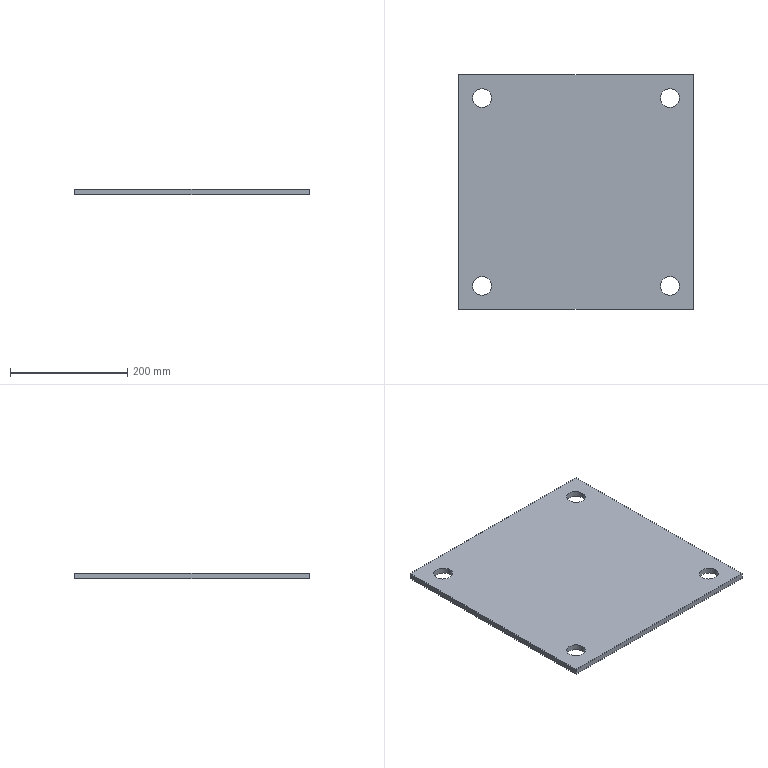Part | SolidWorks | features Extrusion 1 | 1 solid | 14 faces | box 400 x 400 x 10 mm | volume 1567830 mm3 | cylinder 8 | plane 6 | commonest cylinder face diameters 32 x8
STEP:
#1=CARTESIAN_POINT('',(-176.,-160.,10.));
#2=VERTEX_POINT('',#1);
#3=CARTESIAN_POINT('',(-144.,-160.,10.));
#4=VERTEX_POINT('',#3);
#5=CARTESIAN_POINT('',(-160.,-160.,10.));
#6=DIRECTION('',(0.,0.,1.));
#7=DIRECTION('',(1.,0.,0.));
#8=AXIS2_PLACEMENT_3D('',#5,#6,#7);
#9=CIRCLE('',#8,16.);
#10=EDGE_CURVE('',#2,#4,#9,.T.);
#11=ORIENTED_EDGE('',*,*,#10,.T.);
#12=CARTESIAN_POINT('',(-144.,-160.,0.));
#13=VERTEX_POINT('',#12);
#14=CARTESIAN_POINT('',(-144.,-160.,10.));
#15=DIRECTION('',(0.,0.,-1.));
#16=VECTOR('',#15,1000.);
#17=LINE('',#14,#16);
#18=EDGE_CURVE('',#4,#13,#17,.T.);
#19=ORIENTED_EDGE('',*,*,#18,.T.);
#20=CARTESIAN_POINT('',(-176.,-160.,0.));
#21=VERTEX_POINT('',#20);
#22=CARTESIAN_POINT('',(-160.,-160.,0.));
#23=DIRECTION('',(0.,0.,1.));
#24=DIRECTION('',(1.,0.,0.));
#25=AXIS2_PLACEMENT_3D('',#22,#23,#24);
#26=CIRCLE('',#25,16.);
#27=EDGE_CURVE('',#21,#13,#26,.T.);
#28=ORIENTED_EDGE('',*,*,#27,.F.);
#29=CARTESIAN_POINT('',(-176.,-160.,10.));
#30=DIRECTION('',(0.,0.,-1.));
#31=VECTOR('',#30,1000.);
#32=LINE('',#29,#31);
#33=EDGE_CURVE('',#2,#21,#32,.T.);
#34=ORIENTED_EDGE('',*,*,#33,.F.);
#35=EDGE_LOOP('',(#11,#19,#28,#34));
#36=FACE_OUTER_BOUND('',#35,.T.);
#37=CARTESIAN_POINT('',(-160.,-160.,10.));
#38=DIRECTION('',(0.,0.,-1.));
#39=DIRECTION('',(-1.,0.,0.));
#40=AXIS2_PLACEMENT_3D('',#37,#38,#39);
#41=CYLINDRICAL_SURFACE('',#40,16.);
#42=ADVANCED_FACE('',(#36),#41,.F.);
#43=CARTESIAN_POINT('',(144.,-160.,10.));
#44=VERTEX_POINT('',#43);
#45=CARTESIAN_POINT('',(176.,-160.,10.));
#46=VERTEX_POINT('',#45);
#47=CARTESIAN_POINT('',(160.,-160.,10.));
#48=DIRECTION('',(0.,0.,1.));
#49=DIRECTION('',(1.,0.,0.));
#50=AXIS2_PLACEMENT_3D('',#47,#48,#49);
#51=CIRCLE('',#50,16.);
#52=EDGE_CURVE('',#44,#46,#51,.T.);
#53=ORIENTED_EDGE('',*,*,#52,.T.);
#54=CARTESIAN_POINT('',(176.,-160.,0.));
#55=VERTEX_POINT('',#54);
#56=CARTESIAN_POINT('',(176.,-160.,10.));
#57=DIRECTION('',(0.,0.,-1.));
#58=VECTOR('',#57,1000.);
#59=LINE('',#56,#58);
#60=EDGE_CURVE('',#46,#55,#59,.T.);
#61=ORIENTED_EDGE('',*,*,#60,.T.);
#62=CARTESIAN_POINT('',(144.,-160.,0.));
#63=VERTEX_POINT('',#62);
#64=CARTESIAN_POINT('',(160.,-160.,0.));
#65=DIRECTION('',(0.,0.,1.));
#66=DIRECTION('',(1.,0.,0.));
#67=AXIS2_PLACEMENT_3D('',#64,#65,#66);
#68=CIRCLE('',#67,16.);
#69=EDGE_CURVE('',#63,#55,#68,.T.);
#70=ORIENTED_EDGE('',*,*,#69,.F.);
#71=CARTESIAN_POINT('',(144.,-160.,10.));
#72=DIRECTION('',(0.,0.,-1.));
#73=VECTOR('',#72,1000.);
#74=LINE('',#71,#73);
#75=EDGE_CURVE('',#44,#63,#74,.T.);
#76=ORIENTED_EDGE('',*,*,#75,.F.);
#77=EDGE_LOOP('',(#53,#61,#70,#76));
#78=FACE_OUTER_BOUND('',#77,.T.);
#79=CARTESIAN_POINT('',(160.,-160.,10.));
#80=DIRECTION('',(0.,0.,-1.));
#81=DIRECTION('',(-1.,0.,0.));
#82=AXIS2_PLACEMENT_3D('',#79,#80,#81);
#83=CYLINDRICAL_SURFACE('',#82,16.);
#84=ADVANCED_FACE('',(#78),#83,.F.);
#85=CARTESIAN_POINT('',(144.,160.,10.));
#86=VERTEX_POINT('',#85);
#87=CARTESIAN_POINT('',(176.,160.,10.));
#88=VERTEX_POINT('',#87);
#89=CARTESIAN_POINT('',(160.,160.,10.));
#90=DIRECTION('',(0.,0.,1.));
#91=DIRECTION('',(1.,0.,0.));
#92=AXIS2_PLACEMENT_3D('',#89,#90,#91);
#93=CIRCLE('',#92,16.);
#94=EDGE_CURVE('',#86,#88,#93,.T.);
#95=ORIENTED_EDGE('',*,*,#94,.T.);
#96=CARTESIAN_POINT('',(176.,160.,0.));
#97=VERTEX_POINT('',#96);
#98=CARTESIAN_POINT('',(176.,160.,10.));
#99=DIRECTION('',(0.,0.,-1.));
#100=VECTOR('',#99,1000.);
#101=LINE('',#98,#100);
#102=EDGE_CURVE('',#88,#97,#101,.T.);
#103=ORIENTED_EDGE('',*,*,#102,.T.);
#104=CARTESIAN_POINT('',(144.,160.,0.));
#105=VERTEX_POINT('',#104);
#106=CARTESIAN_POINT('',(160.,160.,0.));
#107=DIRECTION('',(0.,0.,1.));
#108=DIRECTION('',(1.,0.,0.));
#109=AXIS2_PLACEMENT_3D('',#106,#107,#108);
#110=CIRCLE('',#109,16.);
#111=EDGE_CURVE('',#105,#97,#110,.T.);
#112=ORIENTED_EDGE('',*,*,#111,.F.);
#113=CARTESIAN_POINT('',(144.,160.,10.));
#114=DIRECTION('',(0.,0.,-1.));
#115=VECTOR('',#114,1000.);
#116=LINE('',#113,#115);
#117=EDGE_CURVE('',#86,#105,#116,.T.);
#118=ORIENTED_EDGE('',*,*,#117,.F.);
#119=EDGE_LOOP('',(#95,#103,#112,#118));
#120=FACE_OUTER_BOUND('',#119,.T.);
#121=CARTESIAN_POINT('',(160.,160.,10.));
#122=DIRECTION('',(0.,0.,-1.));
#123=DIRECTION('',(-1.,0.,0.));
#124=AXIS2_PLACEMENT_3D('',#121,#122,#123);
#125=CYLINDRICAL_SURFACE('',#124,16.);
#126=ADVANCED_FACE('',(#120),#125,.F.);
#127=CARTESIAN_POINT('',(-176.,160.,10.));
#128=VERTEX_POINT('',#127);
#129=CARTESIAN_POINT('',(-144.,160.,10.));
#130=VERTEX_POINT('',#129);
#131=CARTESIAN_POINT('',(-160.,160.,10.));
#132=DIRECTION('',(0.,0.,1.));
#133=DIRECTION('',(1.,0.,0.));
#134=AXIS2_PLACEMENT_3D('',#131,#132,#133);
#135=CIRCLE('',#134,16.);
#136=EDGE_CURVE('',#128,#130,#135,.T.);
#137=ORIENTED_EDGE('',*,*,#136,.T.);
#138=CARTESIAN_POINT('',(-144.,160.,0.));
#139=VERTEX_POINT('',#138);
#140=CARTESIAN_POINT('',(-144.,160.,10.));
#141=DIRECTION('',(0.,0.,-1.));
#142=VECTOR('',#141,1000.);
#143=LINE('',#140,#142);
#144=EDGE_CURVE('',#130,#139,#143,.T.);
#145=ORIENTED_EDGE('',*,*,#144,.T.);
#146=CARTESIAN_POINT('',(-176.,160.,0.));
#147=VERTEX_POINT('',#146);
#148=CARTESIAN_POINT('',(-160.,160.,0.));
#149=DIRECTION('',(0.,0.,1.));
#150=DIRECTION('',(1.,0.,0.));
#151=AXIS2_PLACEMENT_3D('',#148,#149,#150);
#152=CIRCLE('',#151,16.);
#153=EDGE_CURVE('',#147,#139,#152,.T.);
#154=ORIENTED_EDGE('',*,*,#153,.F.);
#155=CARTESIAN_POINT('',(-176.,160.,10.));
#156=DIRECTION('',(0.,0.,-1.));
#157=VECTOR('',#156,1000.);
#158=LINE('',#155,#157);
#159=EDGE_CURVE('',#128,#147,#158,.T.);
#160=ORIENTED_EDGE('',*,*,#159,.F.);
#161=EDGE_LOOP('',(#137,#145,#154,#160));
#162=FACE_OUTER_BOUND('',#161,.T.);
#163=CARTESIAN_POINT('',(-160.,160.,10.));
#164=DIRECTION('',(0.,0.,-1.));
#165=DIRECTION('',(-1.,0.,0.));
#166=AXIS2_PLACEMENT_3D('',#163,#164,#165);
#167=CYLINDRICAL_SURFACE('',#166,16.);
#168=ADVANCED_FACE('',(#162),#167,.F.);
#169=ORIENTED_EDGE('',*,*,#52,.F.);
#170=CARTESIAN_POINT('',(160.,-160.,10.));
#171=DIRECTION('',(0.,0.,1.));
#172=DIRECTION('',(1.,0.,0.));
#173=AXIS2_PLACEMENT_3D('',#170,#171,#172);
#174=CIRCLE('',#173,16.);
#175=EDGE_CURVE('',#46,#44,#174,.T.);
#176=ORIENTED_EDGE('',*,*,#175,.F.);
#177=EDGE_LOOP('',(#169,#176));
#178=FACE_BOUND('',#177,.T.);
#179=ORIENTED_EDGE('',*,*,#136,.F.);
#180=CARTESIAN_POINT('',(-160.,160.,10.));
#181=DIRECTION('',(0.,0.,1.));
#182=DIRECTION('',(1.,0.,0.));
#183=AXIS2_PLACEMENT_3D('',#180,#181,#182);
#184=CIRCLE('',#183,16.);
#185=EDGE_CURVE('',#130,#128,#184,.T.);
#186=ORIENTED_EDGE('',*,*,#185,.F.);
#187=EDGE_LOOP('',(#179,#186));
#188=FACE_BOUND('',#187,.T.);
#189=CARTESIAN_POINT('',(200.,-200.,10.));
#190=VERTEX_POINT('',#189);
#191=CARTESIAN_POINT('',(200.,200.,10.));
#192=VERTEX_POINT('',#191);
#193=CARTESIAN_POINT('',(200.,200.,10.));
#194=DIRECTION('',(0.,1.,0.));
#195=VECTOR('',#194,1000.);
#196=LINE('',#193,#195);
#197=EDGE_CURVE('',#190,#192,#196,.T.);
#198=ORIENTED_EDGE('',*,*,#197,.T.);
#199=CARTESIAN_POINT('',(-200.,200.,10.));
#200=VERTEX_POINT('',#199);
#201=CARTESIAN_POINT('',(-200.,200.,10.));
#202=DIRECTION('',(-1.,0.,0.));
#203=VECTOR('',#202,1000.);
#204=LINE('',#201,#203);
#205=EDGE_CURVE('',#192,#200,#204,.T.);
#206=ORIENTED_EDGE('',*,*,#205,.T.);
#207=CARTESIAN_POINT('',(-200.,-200.,10.));
#208=VERTEX_POINT('',#207);
#209=CARTESIAN_POINT('',(-200.,200.,10.));
#210=DIRECTION('',(0.,-1.,0.));
#211=VECTOR('',#210,1000.);
#212=LINE('',#209,#211);
#213=EDGE_CURVE('',#200,#208,#212,.T.);
#214=ORIENTED_EDGE('',*,*,#213,.T.);
#215=CARTESIAN_POINT('',(-200.,-200.,10.));
#216=DIRECTION('',(1.,0.,0.));
#217=VECTOR('',#216,1000.);
#218=LINE('',#215,#217);
#219=EDGE_CURVE('',#208,#190,#218,.T.);
#220=ORIENTED_EDGE('',*,*,#219,.T.);
#221=EDGE_LOOP('',(#198,#206,#214,#220));
#222=FACE_OUTER_BOUND('',#221,.T.);
#223=ORIENTED_EDGE('',*,*,#94,.F.);
#224=CARTESIAN_POINT('',(160.,160.,10.));
#225=DIRECTION('',(0.,0.,1.));
#226=DIRECTION('',(1.,0.,0.));
#227=AXIS2_PLACEMENT_3D('',#224,#225,#226);
#228=CIRCLE('',#227,16.);
#229=EDGE_CURVE('',#88,#86,#228,.T.);
#230=ORIENTED_EDGE('',*,*,#229,.F.);
#231=EDGE_LOOP('',(#223,#230));
#232=FACE_BOUND('',#231,.T.);
#233=ORIENTED_EDGE('',*,*,#10,.F.);
#234=CARTESIAN_POINT('',(-160.,-160.,10.));
#235=DIRECTION('',(0.,0.,1.));
#236=DIRECTION('',(1.,0.,0.));
#237=AXIS2_PLACEMENT_3D('',#234,#235,#236);
#238=CIRCLE('',#237,16.);
#239=EDGE_CURVE('',#4,#2,#238,.T.);
#240=ORIENTED_EDGE('',*,*,#239,.F.);
#241=EDGE_LOOP('',(#233,#240));
#242=FACE_BOUND('',#241,.T.);
#243=CARTESIAN_POINT('',(0.,0.,10.));
#244=DIRECTION('',(0.,0.,1.));
#245=DIRECTION('',(1.,0.,0.));
#246=AXIS2_PLACEMENT_3D('',#243,#244,#245);
#247=PLANE('',#246);
#248=ADVANCED_FACE('',(#178,#188,#222,#232,#242),#247,.T.);
#249=CARTESIAN_POINT('',(200.,-200.,0.));
#250=VERTEX_POINT('',#249);
#251=CARTESIAN_POINT('',(200.,200.,0.));
#252=VERTEX_POINT('',#251);
#253=CARTESIAN_POINT('',(200.,200.,0.));
#254=DIRECTION('',(0.,1.,0.));
#255=VECTOR('',#254,1000.);
#256=LINE('',#253,#255);
#257=EDGE_CURVE('',#250,#252,#256,.T.);
#258=ORIENTED_EDGE('',*,*,#257,.F.);
#259=CARTESIAN_POINT('',(-200.,-200.,0.));
#260=VERTEX_POINT('',#259);
#261=CARTESIAN_POINT('',(-200.,-200.,0.));
#262=DIRECTION('',(1.,0.,0.));
#263=VECTOR('',#262,1000.);
#264=LINE('',#261,#263);
#265=EDGE_CURVE('',#260,#250,#264,.T.);
#266=ORIENTED_EDGE('',*,*,#265,.F.);
#267=CARTESIAN_POINT('',(-200.,200.,0.));
#268=VERTEX_POINT('',#267);
#269=CARTESIAN_POINT('',(-200.,200.,0.));
#270=DIRECTION('',(0.,-1.,0.));
#271=VECTOR('',#270,1000.);
#272=LINE('',#269,#271);
#273=EDGE_CURVE('',#268,#260,#272,.T.);
#274=ORIENTED_EDGE('',*,*,#273,.F.);
#275=CARTESIAN_POINT('',(-200.,200.,0.));
#276=DIRECTION('',(-1.,0.,0.));
#277=VECTOR('',#276,1000.);
#278=LINE('',#275,#277);
#279=EDGE_CURVE('',#252,#268,#278,.T.);
#280=ORIENTED_EDGE('',*,*,#279,.F.);
#281=EDGE_LOOP('',(#258,#266,#274,#280));
#282=FACE_OUTER_BOUND('',#281,.T.);
#283=ORIENTED_EDGE('',*,*,#153,.T.);
#284=CARTESIAN_POINT('',(-160.,160.,0.));
#285=DIRECTION('',(0.,0.,1.));
#286=DIRECTION('',(1.,0.,0.));
#287=AXIS2_PLACEMENT_3D('',#284,#285,#286);
#288=CIRCLE('',#287,16.);
#289=EDGE_CURVE('',#139,#147,#288,.T.);
#290=ORIENTED_EDGE('',*,*,#289,.T.);
#291=EDGE_LOOP('',(#283,#290));
#292=FACE_BOUND('',#291,.T.);
#293=ORIENTED_EDGE('',*,*,#111,.T.);
#294=CARTESIAN_POINT('',(160.,160.,0.));
#295=DIRECTION('',(0.,0.,1.));
#296=DIRECTION('',(1.,0.,0.));
#297=AXIS2_PLACEMENT_3D('',#294,#295,#296);
#298=CIRCLE('',#297,16.);
#299=EDGE_CURVE('',#97,#105,#298,.T.);
#300=ORIENTED_EDGE('',*,*,#299,.T.);
#301=EDGE_LOOP('',(#293,#300));
#302=FACE_BOUND('',#301,.T.);
#303=ORIENTED_EDGE('',*,*,#69,.T.);
#304=CARTESIAN_POINT('',(160.,-160.,0.));
#305=DIRECTION('',(0.,0.,1.));
#306=DIRECTION('',(1.,0.,0.));
#307=AXIS2_PLACEMENT_3D('',#304,#305,#306);
#308=CIRCLE('',#307,16.);
#309=EDGE_CURVE('',#55,#63,#308,.T.);
#310=ORIENTED_EDGE('',*,*,#309,.T.);
#311=EDGE_LOOP('',(#303,#310));
#312=FACE_BOUND('',#311,.T.);
#313=ORIENTED_EDGE('',*,*,#27,.T.);
#314=CARTESIAN_POINT('',(-160.,-160.,0.));
#315=DIRECTION('',(0.,0.,1.));
#316=DIRECTION('',(1.,0.,0.));
#317=AXIS2_PLACEMENT_3D('',#314,#315,#316);
#318=CIRCLE('',#317,16.);
#319=EDGE_CURVE('',#13,#21,#318,.T.);
#320=ORIENTED_EDGE('',*,*,#319,.T.);
#321=EDGE_LOOP('',(#313,#320));
#322=FACE_BOUND('',#321,.T.);
#323=CARTESIAN_POINT('',(0.,0.,0.));
#324=DIRECTION('',(0.,0.,1.));
#325=DIRECTION('',(1.,0.,0.));
#326=AXIS2_PLACEMENT_3D('',#323,#324,#325);
#327=PLANE('',#326);
#328=ADVANCED_FACE('',(#282,#292,#302,#312,#322),#327,.F.);
#329=ORIENTED_EDGE('',*,*,#257,.T.);
#330=CARTESIAN_POINT('',(200.,200.,10.));
#331=DIRECTION('',(0.,0.,-1.));
#332=VECTOR('',#331,1000.);
#333=LINE('',#330,#332);
#334=EDGE_CURVE('',#192,#252,#333,.T.);
#335=ORIENTED_EDGE('',*,*,#334,.F.);
#336=ORIENTED_EDGE('',*,*,#197,.F.);
#337=CARTESIAN_POINT('',(200.,-200.,10.));
#338=DIRECTION('',(0.,0.,-1.));
#339=VECTOR('',#338,1000.);
#340=LINE('',#337,#339);
#341=EDGE_CURVE('',#190,#250,#340,.T.);
#342=ORIENTED_EDGE('',*,*,#341,.T.);
#343=EDGE_LOOP('',(#329,#335,#336,#342));
#344=FACE_OUTER_BOUND('',#343,.T.);
#345=CARTESIAN_POINT('',(200.,200.,10.));
#346=DIRECTION('',(-1.,0.,0.));
#347=DIRECTION('',(0.,-1.,0.));
#348=AXIS2_PLACEMENT_3D('',#345,#346,#347);
#349=PLANE('',#348);
#350=ADVANCED_FACE('',(#344),#349,.F.);
#351=ORIENTED_EDGE('',*,*,#279,.T.);
#352=CARTESIAN_POINT('',(-200.,200.,10.));
#353=DIRECTION('',(0.,0.,-1.));
#354=VECTOR('',#353,1000.);
#355=LINE('',#352,#354);
#356=EDGE_CURVE('',#200,#268,#355,.T.);
#357=ORIENTED_EDGE('',*,*,#356,.F.);
#358=ORIENTED_EDGE('',*,*,#205,.F.);
#359=ORIENTED_EDGE('',*,*,#334,.T.);
#360=EDGE_LOOP('',(#351,#357,#358,#359));
#361=FACE_OUTER_BOUND('',#360,.T.);
#362=CARTESIAN_POINT('',(-200.,200.,10.));
#363=DIRECTION('',(0.,-1.,0.));
#364=DIRECTION('',(0.,0.,-1.));
#365=AXIS2_PLACEMENT_3D('',#362,#363,#364);
#366=PLANE('',#365);
#367=ADVANCED_FACE('',(#361),#366,.F.);
#368=ORIENTED_EDGE('',*,*,#273,.T.);
#369=CARTESIAN_POINT('',(-200.,-200.,10.));
#370=DIRECTION('',(0.,0.,-1.));
#371=VECTOR('',#370,1000.);
#372=LINE('',#369,#371);
#373=EDGE_CURVE('',#208,#260,#372,.T.);
#374=ORIENTED_EDGE('',*,*,#373,.F.);
#375=ORIENTED_EDGE('',*,*,#213,.F.);
#376=ORIENTED_EDGE('',*,*,#356,.T.);
#377=EDGE_LOOP('',(#368,#374,#375,#376));
#378=FACE_OUTER_BOUND('',#377,.T.);
#379=CARTESIAN_POINT('',(-200.,200.,10.));
#380=DIRECTION('',(1.,0.,0.));
#381=DIRECTION('',(0.,1.,0.));
#382=AXIS2_PLACEMENT_3D('',#379,#380,#381);
#383=PLANE('',#382);
#384=ADVANCED_FACE('',(#378),#383,.F.);
#385=ORIENTED_EDGE('',*,*,#265,.T.);
#386=ORIENTED_EDGE('',*,*,#341,.F.);
#387=ORIENTED_EDGE('',*,*,#219,.F.);
#388=ORIENTED_EDGE('',*,*,#373,.T.);
#389=EDGE_LOOP('',(#385,#386,#387,#388));
#390=FACE_OUTER_BOUND('',#389,.T.);
#391=CARTESIAN_POINT('',(-200.,-200.,10.));
#392=DIRECTION('',(0.,1.,0.));
#393=DIRECTION('',(0.,0.,1.));
#394=AXIS2_PLACEMENT_3D('',#391,#392,#393);
#395=PLANE('',#394);
#396=ADVANCED_FACE('',(#390),#395,.F.);
#397=ORIENTED_EDGE('',*,*,#144,.F.);
#398=ORIENTED_EDGE('',*,*,#185,.T.);
#399=ORIENTED_EDGE('',*,*,#159,.T.);
#400=ORIENTED_EDGE('',*,*,#289,.F.);
#401=EDGE_LOOP('',(#397,#398,#399,#400));
#402=FACE_OUTER_BOUND('',#401,.T.);
#403=CARTESIAN_POINT('',(-160.,160.,10.));
#404=DIRECTION('',(0.,0.,-1.));
#405=DIRECTION('',(-1.,0.,0.));
#406=AXIS2_PLACEMENT_3D('',#403,#404,#405);
#407=CYLINDRICAL_SURFACE('',#406,16.);
#408=ADVANCED_FACE('',(#402),#407,.F.);
#409=ORIENTED_EDGE('',*,*,#102,.F.);
#410=ORIENTED_EDGE('',*,*,#229,.T.);
#411=ORIENTED_EDGE('',*,*,#117,.T.);
#412=ORIENTED_EDGE('',*,*,#299,.F.);
#413=EDGE_LOOP('',(#409,#410,#411,#412));
#414=FACE_OUTER_BOUND('',#413,.T.);
#415=CARTESIAN_POINT('',(160.,160.,10.));
#416=DIRECTION('',(0.,0.,-1.));
#417=DIRECTION('',(-1.,0.,0.));
#418=AXIS2_PLACEMENT_3D('',#415,#416,#417);
#419=CYLINDRICAL_SURFACE('',#418,16.);
#420=ADVANCED_FACE('',(#414),#419,.F.);
#421=ORIENTED_EDGE('',*,*,#60,.F.);
#422=ORIENTED_EDGE('',*,*,#175,.T.);
#423=ORIENTED_EDGE('',*,*,#75,.T.);
#424=ORIENTED_EDGE('',*,*,#309,.F.);
#425=EDGE_LOOP('',(#421,#422,#423,#424));
#426=FACE_OUTER_BOUND('',#425,.T.);
#427=CARTESIAN_POINT('',(160.,-160.,10.));
#428=DIRECTION('',(0.,0.,-1.));
#429=DIRECTION('',(-1.,0.,0.));
#430=AXIS2_PLACEMENT_3D('',#427,#428,#429);
#431=CYLINDRICAL_SURFACE('',#430,16.);
#432=ADVANCED_FACE('',(#426),#431,.F.);
#433=ORIENTED_EDGE('',*,*,#18,.F.);
#434=ORIENTED_EDGE('',*,*,#239,.T.);
#435=ORIENTED_EDGE('',*,*,#33,.T.);
#436=ORIENTED_EDGE('',*,*,#319,.F.);
#437=EDGE_LOOP('',(#433,#434,#435,#436));
#438=FACE_OUTER_BOUND('',#437,.T.);
#439=CARTESIAN_POINT('',(-160.,-160.,10.));
#440=DIRECTION('',(0.,0.,-1.));
#441=DIRECTION('',(-1.,0.,0.));
#442=AXIS2_PLACEMENT_3D('',#439,#440,#441);
#443=CYLINDRICAL_SURFACE('',#442,16.);
#444=ADVANCED_FACE('',(#438),#443,.F.);
#445=CLOSED_SHELL('',(#42,#84,#126,#168,#248,#328,#350,#367,#384,#396,#408,#420,#432,#444));
#446=MANIFOLD_SOLID_BREP('',#445);
#447=CARTESIAN_POINT('',(0.,0.,0.));
#448=DIRECTION('',(0.,0.,1.));
#449=DIRECTION('',(1.,0.,0.));
#450=AXIS2_PLACEMENT_3D('',#447,#448,#449);
#451=(LENGTH_UNIT()NAMED_UNIT(*)SI_UNIT(.MILLI.,.METRE.));
#452=UNCERTAINTY_MEASURE_WITH_UNIT(LENGTH_MEASURE(0.00001),#451,'','');
#453=(NAMED_UNIT(*)PLANE_ANGLE_UNIT()SI_UNIT($,.RADIAN.));
#454=(NAMED_UNIT(*)SI_UNIT($,.STERADIAN.)SOLID_ANGLE_UNIT());
#455=(GEOMETRIC_REPRESENTATION_CONTEXT(3)GLOBAL_UNCERTAINTY_ASSIGNED_CONTEXT((#452))GLOBAL_UNIT_ASSIGNED_CONTEXT((#451,#453,#454))REPRESENTATION_CONTEXT('',''));
#456=ADVANCED_BREP_SHAPE_REPRESENTATION('',(#446,#450),#455);